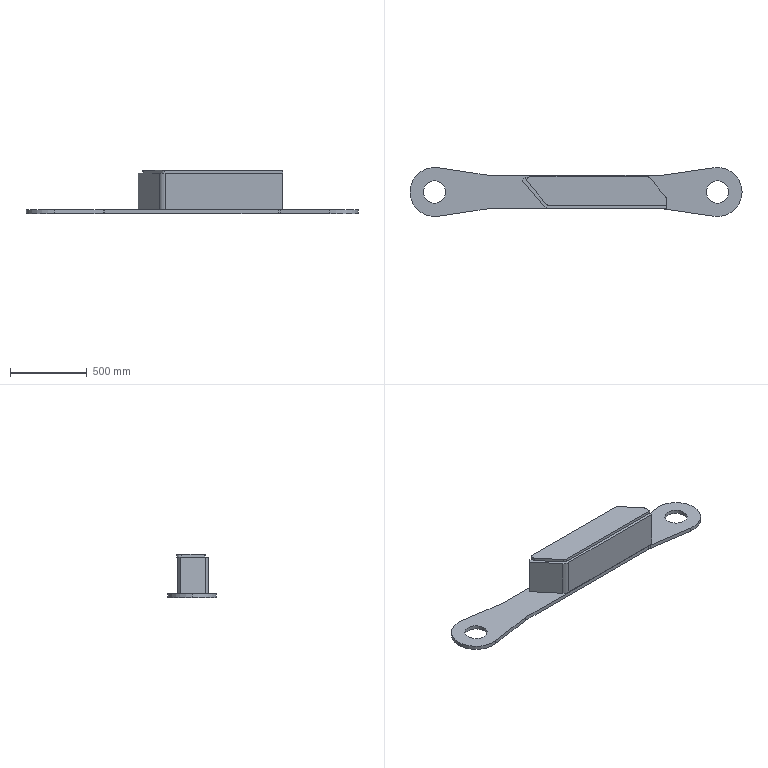Part | NX | features 后连杆右 2 | 1 solid | 48 faces | box 2165 x 320 x 280.474 mm | volume 23006049 mm3 | plane 33 | cylinder 15 | commonest cylinder face diameters 40 x4 200 x4 145 x2 320.239 x2 49.536 x1 100 x1